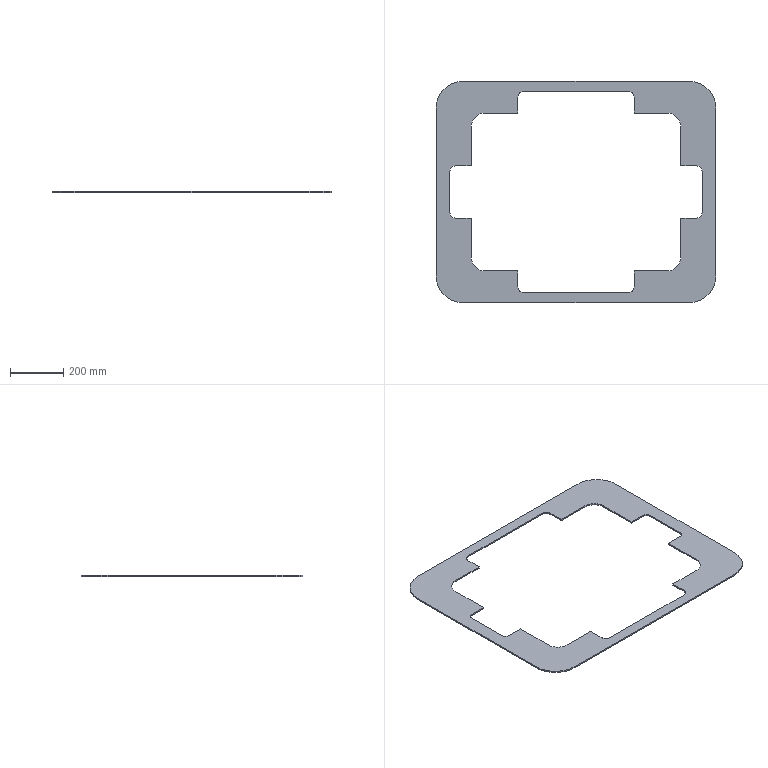Part | NX | features BREP 1 | 1 solid | 42 faces | box 1050 x 830 x 5 mm | volume 1500882 mm3 | plane 26 | cylinder 16 | commonest cylinder face diameters 40 x8 100 x4 200 x4
STEP:
#1=CARTESIAN_POINT('',(817.695,560.835,5.));
#2=VERTEX_POINT('',#1);
#3=CARTESIAN_POINT('',(817.695,560.835,0.));
#4=VERTEX_POINT('',#3);
#5=CARTESIAN_POINT('',(817.695,560.835,44.));
#6=DIRECTION('',(0.,0.,-1.));
#7=VECTOR('',#6,1000.);
#8=LINE('',#5,#7);
#9=EDGE_CURVE('',#2,#4,#8,.T.);
#10=ORIENTED_EDGE('',*,*,#9,.T.);
#11=CARTESIAN_POINT('',(817.695,412.627,0.));
#12=VERTEX_POINT('',#11);
#13=CARTESIAN_POINT('',(817.695,630.,0.));
#14=DIRECTION('',(0.,1.,0.));
#15=VECTOR('',#14,1000.);
#16=LINE('',#13,#15);
#17=EDGE_CURVE('',#12,#4,#16,.T.);
#18=ORIENTED_EDGE('',*,*,#17,.F.);
#19=CARTESIAN_POINT('',(817.695,412.627,5.));
#20=VERTEX_POINT('',#19);
#21=CARTESIAN_POINT('',(817.695,412.627,44.));
#22=DIRECTION('',(0.,0.,-1.));
#23=VECTOR('',#22,1000.);
#24=LINE('',#21,#23);
#25=EDGE_CURVE('',#20,#12,#24,.T.);
#26=ORIENTED_EDGE('',*,*,#25,.F.);
#27=CARTESIAN_POINT('',(817.695,630.,5.));
#28=DIRECTION('',(0.,-1.,0.));
#29=VECTOR('',#28,1000.);
#30=LINE('',#27,#29);
#31=EDGE_CURVE('',#2,#20,#30,.T.);
#32=ORIENTED_EDGE('',*,*,#31,.F.);
#33=EDGE_LOOP('',(#10,#18,#26,#32));
#34=FACE_BOUND('',#33,.T.);
#35=CARTESIAN_POINT('',(817.695,467.627,44.));
#36=DIRECTION('',(-1.,0.,0.));
#37=DIRECTION('',(0.,-1.,0.));
#38=AXIS2_PLACEMENT_3D('',#35,#36,#37);
#39=PLANE('',#38);
#40=ADVANCED_FACE('',(#34),#39,.T.);
#41=CARTESIAN_POINT('',(642.627,610.835,0.));
#42=VERTEX_POINT('',#41);
#43=CARTESIAN_POINT('',(642.627,610.835,5.));
#44=VERTEX_POINT('',#43);
#45=CARTESIAN_POINT('',(642.627,610.835,44.));
#46=DIRECTION('',(0.,0.,1.));
#47=VECTOR('',#46,1000.);
#48=LINE('',#45,#47);
#49=EDGE_CURVE('',#42,#44,#48,.T.);
#50=ORIENTED_EDGE('',*,*,#49,.F.);
#51=CARTESIAN_POINT('',(767.695,610.835,0.));
#52=VERTEX_POINT('',#51);
#53=CARTESIAN_POINT('',(850.,610.835,0.));
#54=DIRECTION('',(-1.,0.,0.));
#55=VECTOR('',#54,1000.);
#56=LINE('',#53,#55);
#57=EDGE_CURVE('',#52,#42,#56,.T.);
#58=ORIENTED_EDGE('',*,*,#57,.F.);
#59=CARTESIAN_POINT('',(767.695,610.835,5.));
#60=VERTEX_POINT('',#59);
#61=CARTESIAN_POINT('',(767.695,610.835,44.));
#62=DIRECTION('',(0.,0.,-1.));
#63=VECTOR('',#62,1000.);
#64=LINE('',#61,#63);
#65=EDGE_CURVE('',#60,#52,#64,.T.);
#66=ORIENTED_EDGE('',*,*,#65,.F.);
#67=CARTESIAN_POINT('',(850.,610.835,5.));
#68=DIRECTION('',(1.,0.,0.));
#69=VECTOR('',#68,1000.);
#70=LINE('',#67,#69);
#71=EDGE_CURVE('',#44,#60,#70,.T.);
#72=ORIENTED_EDGE('',*,*,#71,.F.);
#73=EDGE_LOOP('',(#50,#58,#66,#72));
#74=FACE_BOUND('',#73,.T.);
#75=CARTESIAN_POINT('',(687.627,610.835,44.));
#76=DIRECTION('',(0.,-1.,0.));
#77=DIRECTION('',(1.,0.,0.));
#78=AXIS2_PLACEMENT_3D('',#75,#76,#77);
#79=PLANE('',#78);
#80=ADVANCED_FACE('',(#74),#79,.T.);
#81=ORIENTED_EDGE('',*,*,#65,.T.);
#82=CARTESIAN_POINT('',(767.695,560.835,0.));
#83=DIRECTION('',(0.,0.,1.));
#84=DIRECTION('',(-1.,0.,0.));
#85=AXIS2_PLACEMENT_3D('',#82,#83,#84);
#86=CIRCLE('',#85,50.);
#87=EDGE_CURVE('',#4,#52,#86,.T.);
#88=ORIENTED_EDGE('',*,*,#87,.F.);
#89=ORIENTED_EDGE('',*,*,#9,.F.);
#90=CARTESIAN_POINT('',(767.695,560.835,5.));
#91=DIRECTION('',(0.,0.,1.));
#92=DIRECTION('',(-1.,0.,0.));
#93=AXIS2_PLACEMENT_3D('',#90,#91,#92);
#94=CIRCLE('',#93,50.);
#95=EDGE_CURVE('',#2,#60,#94,.T.);
#96=ORIENTED_EDGE('',*,*,#95,.T.);
#97=EDGE_LOOP('',(#81,#88,#89,#96));
#98=FACE_BOUND('',#97,.T.);
#99=CARTESIAN_POINT('',(767.695,560.835,44.));
#100=DIRECTION('',(0.,0.,-1.));
#101=DIRECTION('',(-1.,0.,0.));
#102=AXIS2_PLACEMENT_3D('',#99,#100,#101);
#103=CYLINDRICAL_SURFACE('',#102,50.);
#104=ADVANCED_FACE('',(#98),#103,.F.);
#105=CARTESIAN_POINT('',(642.627,-40.835,0.));
#106=VERTEX_POINT('',#105);
#107=CARTESIAN_POINT('',(642.627,19.165,0.));
#108=VERTEX_POINT('',#107);
#109=CARTESIAN_POINT('',(642.627,-60.835,0.));
#110=DIRECTION('',(0.,1.,0.));
#111=VECTOR('',#110,1000.);
#112=LINE('',#109,#111);
#113=EDGE_CURVE('',#106,#108,#112,.T.);
#114=ORIENTED_EDGE('',*,*,#113,.F.);
#115=CARTESIAN_POINT('',(642.627,-40.835,5.));
#116=VERTEX_POINT('',#115);
#117=CARTESIAN_POINT('',(642.627,-40.835,5.));
#118=DIRECTION('',(0.,0.,1.));
#119=VECTOR('',#118,1000.);
#120=LINE('',#117,#119);
#121=EDGE_CURVE('',#106,#116,#120,.T.);
#122=ORIENTED_EDGE('',*,*,#121,.T.);
#123=CARTESIAN_POINT('',(642.627,19.165,5.));
#124=VERTEX_POINT('',#123);
#125=CARTESIAN_POINT('',(642.627,-60.835,5.));
#126=DIRECTION('',(0.,1.,0.));
#127=VECTOR('',#126,1000.);
#128=LINE('',#125,#127);
#129=EDGE_CURVE('',#116,#124,#128,.T.);
#130=ORIENTED_EDGE('',*,*,#129,.T.);
#131=CARTESIAN_POINT('',(642.627,19.165,44.));
#132=DIRECTION('',(0.,0.,-1.));
#133=VECTOR('',#132,1000.);
#134=LINE('',#131,#133);
#135=EDGE_CURVE('',#124,#108,#134,.T.);
#136=ORIENTED_EDGE('',*,*,#135,.T.);
#137=EDGE_LOOP('',(#114,#122,#130,#136));
#138=FACE_BOUND('',#137,.T.);
#139=CARTESIAN_POINT('',(642.627,-60.835,0.));
#140=DIRECTION('',(1.,0.,0.));
#141=DIRECTION('',(0.,-1.,0.));
#142=AXIS2_PLACEMENT_3D('',#139,#140,#141);
#143=PLANE('',#142);
#144=ADVANCED_FACE('',(#138),#143,.F.);
#145=CARTESIAN_POINT('',(227.373,-60.835,5.));
#146=VERTEX_POINT('',#145);
#147=CARTESIAN_POINT('',(622.627,-60.835,5.));
#148=VERTEX_POINT('',#147);
#149=CARTESIAN_POINT('',(167.373,-60.835,5.));
#150=DIRECTION('',(1.,0.,0.));
#151=VECTOR('',#150,1000.);
#152=LINE('',#149,#151);
#153=EDGE_CURVE('',#146,#148,#152,.T.);
#154=ORIENTED_EDGE('',*,*,#153,.T.);
#155=CARTESIAN_POINT('',(622.627,-60.835,0.));
#156=VERTEX_POINT('',#155);
#157=CARTESIAN_POINT('',(622.627,-60.835,0.));
#158=DIRECTION('',(0.,0.,-1.));
#159=VECTOR('',#158,1000.);
#160=LINE('',#157,#159);
#161=EDGE_CURVE('',#148,#156,#160,.T.);
#162=ORIENTED_EDGE('',*,*,#161,.T.);
#163=CARTESIAN_POINT('',(227.373,-60.835,0.));
#164=VERTEX_POINT('',#163);
#165=CARTESIAN_POINT('',(167.373,-60.835,0.));
#166=DIRECTION('',(1.,0.,0.));
#167=VECTOR('',#166,1000.);
#168=LINE('',#165,#167);
#169=EDGE_CURVE('',#164,#156,#168,.T.);
#170=ORIENTED_EDGE('',*,*,#169,.F.);
#171=CARTESIAN_POINT('',(227.373,-60.835,5.));
#172=DIRECTION('',(0.,0.,1.));
#173=VECTOR('',#172,1000.);
#174=LINE('',#171,#173);
#175=EDGE_CURVE('',#164,#146,#174,.T.);
#176=ORIENTED_EDGE('',*,*,#175,.T.);
#177=EDGE_LOOP('',(#154,#162,#170,#176));
#178=FACE_BOUND('',#177,.T.);
#179=CARTESIAN_POINT('',(167.373,-60.835,0.));
#180=DIRECTION('',(0.,-1.,0.));
#181=DIRECTION('',(-1.,0.,0.));
#182=AXIS2_PLACEMENT_3D('',#179,#180,#181);
#183=PLANE('',#182);
#184=ADVANCED_FACE('',(#178),#183,.F.);
#185=CARTESIAN_POINT('',(207.373,19.165,5.));
#186=VERTEX_POINT('',#185);
#187=CARTESIAN_POINT('',(207.373,-40.835,5.));
#188=VERTEX_POINT('',#187);
#189=CARTESIAN_POINT('',(207.373,167.373,5.));
#190=DIRECTION('',(0.,-1.,0.));
#191=VECTOR('',#190,1000.);
#192=LINE('',#189,#191);
#193=EDGE_CURVE('',#186,#188,#192,.T.);
#194=ORIENTED_EDGE('',*,*,#193,.T.);
#195=CARTESIAN_POINT('',(207.373,-40.835,0.));
#196=VERTEX_POINT('',#195);
#197=CARTESIAN_POINT('',(207.373,-40.835,0.));
#198=DIRECTION('',(0.,0.,-1.));
#199=VECTOR('',#198,1000.);
#200=LINE('',#197,#199);
#201=EDGE_CURVE('',#188,#196,#200,.T.);
#202=ORIENTED_EDGE('',*,*,#201,.T.);
#203=CARTESIAN_POINT('',(207.373,19.165,0.));
#204=VERTEX_POINT('',#203);
#205=CARTESIAN_POINT('',(207.373,167.373,0.));
#206=DIRECTION('',(0.,-1.,0.));
#207=VECTOR('',#206,1000.);
#208=LINE('',#205,#207);
#209=EDGE_CURVE('',#204,#196,#208,.T.);
#210=ORIENTED_EDGE('',*,*,#209,.F.);
#211=CARTESIAN_POINT('',(207.373,19.165,44.));
#212=DIRECTION('',(0.,0.,1.));
#213=VECTOR('',#212,1000.);
#214=LINE('',#211,#213);
#215=EDGE_CURVE('',#204,#186,#214,.T.);
#216=ORIENTED_EDGE('',*,*,#215,.T.);
#217=EDGE_LOOP('',(#194,#202,#210,#216));
#218=FACE_BOUND('',#217,.T.);
#219=CARTESIAN_POINT('',(207.373,167.373,0.));
#220=DIRECTION('',(-1.,0.,0.));
#221=DIRECTION('',(0.,1.,0.));
#222=AXIS2_PLACEMENT_3D('',#219,#220,#221);
#223=PLANE('',#222);
#224=ADVANCED_FACE('',(#218),#223,.F.);
#225=ORIENTED_EDGE('',*,*,#215,.F.);
#226=CARTESIAN_POINT('',(82.305,19.165,0.));
#227=VERTEX_POINT('',#226);
#228=CARTESIAN_POINT('',(0.,19.165,0.));
#229=DIRECTION('',(1.,0.,0.));
#230=VECTOR('',#229,1000.);
#231=LINE('',#228,#230);
#232=EDGE_CURVE('',#227,#204,#231,.T.);
#233=ORIENTED_EDGE('',*,*,#232,.F.);
#234=CARTESIAN_POINT('',(82.305,19.165,5.));
#235=VERTEX_POINT('',#234);
#236=CARTESIAN_POINT('',(82.305,19.165,44.));
#237=DIRECTION('',(0.,0.,-1.));
#238=VECTOR('',#237,1000.);
#239=LINE('',#236,#238);
#240=EDGE_CURVE('',#235,#227,#239,.T.);
#241=ORIENTED_EDGE('',*,*,#240,.F.);
#242=CARTESIAN_POINT('',(0.,19.165,5.));
#243=DIRECTION('',(-1.,0.,0.));
#244=VECTOR('',#243,1000.);
#245=LINE('',#242,#244);
#246=EDGE_CURVE('',#186,#235,#245,.T.);
#247=ORIENTED_EDGE('',*,*,#246,.F.);
#248=EDGE_LOOP('',(#225,#233,#241,#247));
#249=FACE_BOUND('',#248,.T.);
#250=CARTESIAN_POINT('',(162.373,19.165,44.));
#251=DIRECTION('',(0.,1.,0.));
#252=DIRECTION('',(-1.,0.,0.));
#253=AXIS2_PLACEMENT_3D('',#250,#251,#252);
#254=PLANE('',#253);
#255=ADVANCED_FACE('',(#249),#254,.T.);
#256=ORIENTED_EDGE('',*,*,#240,.T.);
#257=CARTESIAN_POINT('',(32.305,69.165,0.));
#258=VERTEX_POINT('',#257);
#259=CARTESIAN_POINT('',(82.305,69.165,0.));
#260=DIRECTION('',(0.,0.,1.));
#261=DIRECTION('',(-1.,0.,0.));
#262=AXIS2_PLACEMENT_3D('',#259,#260,#261);
#263=CIRCLE('',#262,50.);
#264=EDGE_CURVE('',#258,#227,#263,.T.);
#265=ORIENTED_EDGE('',*,*,#264,.F.);
#266=CARTESIAN_POINT('',(32.305,69.165,5.));
#267=VERTEX_POINT('',#266);
#268=CARTESIAN_POINT('',(32.305,69.165,44.));
#269=DIRECTION('',(0.,0.,-1.));
#270=VECTOR('',#269,1000.);
#271=LINE('',#268,#270);
#272=EDGE_CURVE('',#267,#258,#271,.T.);
#273=ORIENTED_EDGE('',*,*,#272,.F.);
#274=CARTESIAN_POINT('',(82.305,69.165,5.));
#275=DIRECTION('',(0.,0.,1.));
#276=DIRECTION('',(-1.,0.,0.));
#277=AXIS2_PLACEMENT_3D('',#274,#275,#276);
#278=CIRCLE('',#277,50.);
#279=EDGE_CURVE('',#267,#235,#278,.T.);
#280=ORIENTED_EDGE('',*,*,#279,.T.);
#281=EDGE_LOOP('',(#256,#265,#273,#280));
#282=FACE_BOUND('',#281,.T.);
#283=CARTESIAN_POINT('',(82.305,69.165,44.));
#284=DIRECTION('',(0.,0.,-1.));
#285=DIRECTION('',(1.,0.,0.));
#286=AXIS2_PLACEMENT_3D('',#283,#284,#285);
#287=CYLINDRICAL_SURFACE('',#286,50.);
#288=ADVANCED_FACE('',(#282),#287,.F.);
#289=ORIENTED_EDGE('',*,*,#272,.T.);
#290=CARTESIAN_POINT('',(32.305,217.373,0.));
#291=VERTEX_POINT('',#290);
#292=CARTESIAN_POINT('',(32.305,0.,0.));
#293=DIRECTION('',(0.,-1.,0.));
#294=VECTOR('',#293,1000.);
#295=LINE('',#292,#294);
#296=EDGE_CURVE('',#291,#258,#295,.T.);
#297=ORIENTED_EDGE('',*,*,#296,.F.);
#298=CARTESIAN_POINT('',(32.305,217.373,5.));
#299=VERTEX_POINT('',#298);
#300=CARTESIAN_POINT('',(32.305,217.373,44.));
#301=DIRECTION('',(0.,0.,-1.));
#302=VECTOR('',#301,1000.);
#303=LINE('',#300,#302);
#304=EDGE_CURVE('',#299,#291,#303,.T.);
#305=ORIENTED_EDGE('',*,*,#304,.F.);
#306=CARTESIAN_POINT('',(32.305,0.,5.));
#307=DIRECTION('',(0.,1.,0.));
#308=VECTOR('',#307,1000.);
#309=LINE('',#306,#308);
#310=EDGE_CURVE('',#267,#299,#309,.T.);
#311=ORIENTED_EDGE('',*,*,#310,.F.);
#312=EDGE_LOOP('',(#289,#297,#305,#311));
#313=FACE_BOUND('',#312,.T.);
#314=CARTESIAN_POINT('',(32.305,162.373,44.));
#315=DIRECTION('',(1.,0.,0.));
#316=DIRECTION('',(0.,1.,0.));
#317=AXIS2_PLACEMENT_3D('',#314,#315,#316);
#318=PLANE('',#317);
#319=ADVANCED_FACE('',(#313),#318,.T.);
#320=CARTESIAN_POINT('',(-27.695,217.373,0.));
#321=VERTEX_POINT('',#320);
#322=CARTESIAN_POINT('',(-47.695,217.373,0.));
#323=DIRECTION('',(1.,0.,0.));
#324=VECTOR('',#323,1000.);
#325=LINE('',#322,#324);
#326=EDGE_CURVE('',#321,#291,#325,.T.);
#327=ORIENTED_EDGE('',*,*,#326,.F.);
#328=CARTESIAN_POINT('',(-27.695,217.373,5.));
#329=VERTEX_POINT('',#328);
#330=CARTESIAN_POINT('',(-27.695,217.373,5.));
#331=DIRECTION('',(0.,0.,1.));
#332=VECTOR('',#331,1000.);
#333=LINE('',#330,#332);
#334=EDGE_CURVE('',#321,#329,#333,.T.);
#335=ORIENTED_EDGE('',*,*,#334,.T.);
#336=CARTESIAN_POINT('',(-47.695,217.373,5.));
#337=DIRECTION('',(1.,0.,0.));
#338=VECTOR('',#337,1000.);
#339=LINE('',#336,#338);
#340=EDGE_CURVE('',#329,#299,#339,.T.);
#341=ORIENTED_EDGE('',*,*,#340,.T.);
#342=ORIENTED_EDGE('',*,*,#304,.T.);
#343=EDGE_LOOP('',(#327,#335,#341,#342));
#344=FACE_BOUND('',#343,.T.);
#345=CARTESIAN_POINT('',(-47.695,217.373,0.));
#346=DIRECTION('',(0.,-1.,0.));
#347=DIRECTION('',(-1.,0.,0.));
#348=AXIS2_PLACEMENT_3D('',#345,#346,#347);
#349=PLANE('',#348);
#350=ADVANCED_FACE('',(#344),#349,.F.);
#351=CARTESIAN_POINT('',(-47.695,392.627,0.));
#352=VERTEX_POINT('',#351);
#353=CARTESIAN_POINT('',(-47.695,237.373,0.));
#354=VERTEX_POINT('',#353);
#355=CARTESIAN_POINT('',(-47.695,462.627,0.));
#356=DIRECTION('',(0.,-1.,0.));
#357=VECTOR('',#356,1000.);
#358=LINE('',#355,#357);
#359=EDGE_CURVE('',#352,#354,#358,.T.);
#360=ORIENTED_EDGE('',*,*,#359,.F.);
#361=CARTESIAN_POINT('',(-47.695,392.627,5.));
#362=VERTEX_POINT('',#361);
#363=CARTESIAN_POINT('',(-47.695,392.627,5.));
#364=DIRECTION('',(0.,0.,1.));
#365=VECTOR('',#364,1000.);
#366=LINE('',#363,#365);
#367=EDGE_CURVE('',#352,#362,#366,.T.);
#368=ORIENTED_EDGE('',*,*,#367,.T.);
#369=CARTESIAN_POINT('',(-47.695,237.373,5.));
#370=VERTEX_POINT('',#369);
#371=CARTESIAN_POINT('',(-47.695,462.627,5.));
#372=DIRECTION('',(0.,-1.,0.));
#373=VECTOR('',#372,1000.);
#374=LINE('',#371,#373);
#375=EDGE_CURVE('',#362,#370,#374,.T.);
#376=ORIENTED_EDGE('',*,*,#375,.T.);
#377=CARTESIAN_POINT('',(-47.695,237.373,0.));
#378=DIRECTION('',(0.,0.,-1.));
#379=VECTOR('',#378,1000.);
#380=LINE('',#377,#379);
#381=EDGE_CURVE('',#370,#354,#380,.T.);
#382=ORIENTED_EDGE('',*,*,#381,.T.);
#383=EDGE_LOOP('',(#360,#368,#376,#382));
#384=FACE_BOUND('',#383,.T.);
#385=CARTESIAN_POINT('',(-47.695,462.627,0.));
#386=DIRECTION('',(-1.,0.,0.));
#387=DIRECTION('',(0.,1.,0.));
#388=AXIS2_PLACEMENT_3D('',#385,#386,#387);
#389=PLANE('',#388);
#390=ADVANCED_FACE('',(#384),#389,.F.);
#391=CARTESIAN_POINT('',(32.305,412.627,5.));
#392=VERTEX_POINT('',#391);
#393=CARTESIAN_POINT('',(-27.695,412.627,5.));
#394=VERTEX_POINT('',#393);
#395=CARTESIAN_POINT('',(167.373,412.627,5.));
#396=DIRECTION('',(-1.,0.,0.));
#397=VECTOR('',#396,1000.);
#398=LINE('',#395,#397);
#399=EDGE_CURVE('',#392,#394,#398,.T.);
#400=ORIENTED_EDGE('',*,*,#399,.T.);
#401=CARTESIAN_POINT('',(-27.695,412.627,0.));
#402=VERTEX_POINT('',#401);
#403=CARTESIAN_POINT('',(-27.695,412.627,0.));
#404=DIRECTION('',(0.,0.,-1.));
#405=VECTOR('',#404,1000.);
#406=LINE('',#403,#405);
#407=EDGE_CURVE('',#394,#402,#406,.T.);
#408=ORIENTED_EDGE('',*,*,#407,.T.);
#409=CARTESIAN_POINT('',(32.305,412.627,0.));
#410=VERTEX_POINT('',#409);
#411=CARTESIAN_POINT('',(167.373,412.627,0.));
#412=DIRECTION('',(-1.,0.,0.));
#413=VECTOR('',#412,1000.);
#414=LINE('',#411,#413);
#415=EDGE_CURVE('',#410,#402,#414,.T.);
#416=ORIENTED_EDGE('',*,*,#415,.F.);
#417=CARTESIAN_POINT('',(32.305,412.627,0.));
#418=DIRECTION('',(0.,0.,-1.));
#419=VECTOR('',#418,1000.);
#420=LINE('',#417,#419);
#421=EDGE_CURVE('',#392,#410,#420,.T.);
#422=ORIENTED_EDGE('',*,*,#421,.F.);
#423=EDGE_LOOP('',(#400,#408,#416,#422));
#424=FACE_BOUND('',#423,.T.);
#425=CARTESIAN_POINT('',(167.373,412.627,0.));
#426=DIRECTION('',(0.,1.,0.));
#427=DIRECTION('',(1.,0.,0.));
#428=AXIS2_PLACEMENT_3D('',#425,#426,#427);
#429=PLANE('',#428);
#430=ADVANCED_FACE('',(#424),#429,.F.);
#431=CARTESIAN_POINT('',(32.305,560.835,0.));
#432=VERTEX_POINT('',#431);
#433=CARTESIAN_POINT('',(32.305,560.835,5.));
#434=VERTEX_POINT('',#433);
#435=CARTESIAN_POINT('',(32.305,560.835,44.));
#436=DIRECTION('',(0.,0.,1.));
#437=VECTOR('',#436,1000.);
#438=LINE('',#435,#437);
#439=EDGE_CURVE('',#432,#434,#438,.T.);
#440=ORIENTED_EDGE('',*,*,#439,.T.);
#441=CARTESIAN_POINT('',(32.305,630.,5.));
#442=DIRECTION('',(0.,-1.,0.));
#443=VECTOR('',#442,1000.);
#444=LINE('',#441,#443);
#445=EDGE_CURVE('',#434,#392,#444,.T.);
#446=ORIENTED_EDGE('',*,*,#445,.T.);
#447=ORIENTED_EDGE('',*,*,#421,.T.);
#448=CARTESIAN_POINT('',(32.305,630.,0.));
#449=DIRECTION('',(0.,-1.,0.));
#450=VECTOR('',#449,1000.);
#451=LINE('',#448,#450);
#452=EDGE_CURVE('',#432,#410,#451,.T.);
#453=ORIENTED_EDGE('',*,*,#452,.F.);
#454=EDGE_LOOP('',(#440,#446,#447,#453));
#455=FACE_BOUND('',#454,.T.);
#456=CARTESIAN_POINT('',(32.305,467.627,44.));
#457=DIRECTION('',(1.,0.,0.));
#458=DIRECTION('',(0.,-1.,0.));
#459=AXIS2_PLACEMENT_3D('',#456,#457,#458);
#460=PLANE('',#459);
#461=ADVANCED_FACE('',(#455),#460,.T.);
#462=CARTESIAN_POINT('',(82.305,610.835,0.));
#463=VERTEX_POINT('',#462);
#464=CARTESIAN_POINT('',(82.305,610.835,5.));
#465=VERTEX_POINT('',#464);
#466=CARTESIAN_POINT('',(82.305,610.835,44.));
#467=DIRECTION('',(0.,0.,1.));
#468=VECTOR('',#467,1000.);
#469=LINE('',#466,#468);
#470=EDGE_CURVE('',#463,#465,#469,.T.);
#471=ORIENTED_EDGE('',*,*,#470,.T.);
#472=CARTESIAN_POINT('',(82.305,560.835,5.));
#473=DIRECTION('',(0.,0.,1.));
#474=DIRECTION('',(-1.,0.,0.));
#475=AXIS2_PLACEMENT_3D('',#472,#473,#474);
#476=CIRCLE('',#475,50.);
#477=EDGE_CURVE('',#465,#434,#476,.T.);
#478=ORIENTED_EDGE('',*,*,#477,.T.);
#479=ORIENTED_EDGE('',*,*,#439,.F.);
#480=CARTESIAN_POINT('',(82.305,560.835,0.));
#481=DIRECTION('',(0.,0.,1.));
#482=DIRECTION('',(-1.,0.,0.));
#483=AXIS2_PLACEMENT_3D('',#480,#481,#482);
#484=CIRCLE('',#483,50.);
#485=EDGE_CURVE('',#463,#432,#484,.T.);
#486=ORIENTED_EDGE('',*,*,#485,.F.);
#487=EDGE_LOOP('',(#471,#478,#479,#486));
#488=FACE_BOUND('',#487,.T.);
#489=CARTESIAN_POINT('',(82.305,560.835,44.));
#490=DIRECTION('',(0.,0.,-1.));
#491=DIRECTION('',(1.,0.,0.));
#492=AXIS2_PLACEMENT_3D('',#489,#490,#491);
#493=CYLINDRICAL_SURFACE('',#492,50.);
#494=ADVANCED_FACE('',(#488),#493,.F.);
#495=CARTESIAN_POINT('',(207.373,610.835,0.));
#496=VERTEX_POINT('',#495);
#497=CARTESIAN_POINT('',(207.373,610.835,5.));
#498=VERTEX_POINT('',#497);
#499=CARTESIAN_POINT('',(207.373,610.835,0.));
#500=DIRECTION('',(0.,0.,1.));
#501=VECTOR('',#500,1000.);
#502=LINE('',#499,#501);
#503=EDGE_CURVE('',#496,#498,#502,.T.);
#504=ORIENTED_EDGE('',*,*,#503,.T.);
#505=CARTESIAN_POINT('',(0.,610.835,5.));
#506=DIRECTION('',(-1.,0.,0.));
#507=VECTOR('',#506,1000.);
#508=LINE('',#505,#507);
#509=EDGE_CURVE('',#498,#465,#508,.T.);
#510=ORIENTED_EDGE('',*,*,#509,.T.);
#511=ORIENTED_EDGE('',*,*,#470,.F.);
#512=CARTESIAN_POINT('',(0.,610.835,0.));
#513=DIRECTION('',(-1.,0.,0.));
#514=VECTOR('',#513,1000.);
#515=LINE('',#512,#514);
#516=EDGE_CURVE('',#496,#463,#515,.T.);
#517=ORIENTED_EDGE('',*,*,#516,.F.);
#518=EDGE_LOOP('',(#504,#510,#511,#517));
#519=FACE_BOUND('',#518,.T.);
#520=CARTESIAN_POINT('',(162.373,610.835,44.));
#521=DIRECTION('',(0.,-1.,0.));
#522=DIRECTION('',(-1.,0.,0.));
#523=AXIS2_PLACEMENT_3D('',#520,#521,#522);
#524=PLANE('',#523);
#525=ADVANCED_FACE('',(#519),#524,.T.);
#526=CARTESIAN_POINT('',(207.373,670.835,0.));
#527=VERTEX_POINT('',#526);
#528=CARTESIAN_POINT('',(207.373,690.835,0.));
#529=DIRECTION('',(0.,-1.,0.));
#530=VECTOR('',#529,1000.);
#531=LINE('',#528,#530);
#532=EDGE_CURVE('',#527,#496,#531,.T.);
#533=ORIENTED_EDGE('',*,*,#532,.F.);
#534=CARTESIAN_POINT('',(207.373,670.835,5.));
#535=VERTEX_POINT('',#534);
#536=CARTESIAN_POINT('',(207.373,670.835,5.));
#537=DIRECTION('',(0.,0.,1.));
#538=VECTOR('',#537,1000.);
#539=LINE('',#536,#538);
#540=EDGE_CURVE('',#527,#535,#539,.T.);
#541=ORIENTED_EDGE('',*,*,#540,.T.);
#542=CARTESIAN_POINT('',(207.373,690.835,5.));
#543=DIRECTION('',(0.,-1.,0.));
#544=VECTOR('',#543,1000.);
#545=LINE('',#542,#544);
#546=EDGE_CURVE('',#535,#498,#545,.T.);
#547=ORIENTED_EDGE('',*,*,#546,.T.);
#548=ORIENTED_EDGE('',*,*,#503,.F.);
#549=EDGE_LOOP('',(#533,#541,#547,#548));
#550=FACE_BOUND('',#549,.T.);
#551=CARTESIAN_POINT('',(207.373,690.835,0.));
#552=DIRECTION('',(-1.,0.,0.));
#553=DIRECTION('',(0.,1.,0.));
#554=AXIS2_PLACEMENT_3D('',#551,#552,#553);
#555=PLANE('',#554);
#556=ADVANCED_FACE('',(#550),#555,.F.);
#557=CARTESIAN_POINT('',(622.627,690.835,5.));
#558=VERTEX_POINT('',#557);
#559=CARTESIAN_POINT('',(227.373,690.835,5.));
#560=VERTEX_POINT('',#559);
#561=CARTESIAN_POINT('',(682.627,690.835,5.));
#562=DIRECTION('',(-1.,0.,0.));
#563=VECTOR('',#562,1000.);
#564=LINE('',#561,#563);
#565=EDGE_CURVE('',#558,#560,#564,.T.);
#566=ORIENTED_EDGE('',*,*,#565,.T.);
#567=CARTESIAN_POINT('',(227.373,690.835,0.));
#568=VERTEX_POINT('',#567);
#569=CARTESIAN_POINT('',(227.373,690.835,0.));
#570=DIRECTION('',(0.,0.,-1.));
#571=VECTOR('',#570,1000.);
#572=LINE('',#569,#571);
#573=EDGE_CURVE('',#560,#568,#572,.T.);
#574=ORIENTED_EDGE('',*,*,#573,.T.);
#575=CARTESIAN_POINT('',(622.627,690.835,0.));
#576=VERTEX_POINT('',#575);
#577=CARTESIAN_POINT('',(682.627,690.835,0.));
#578=DIRECTION('',(-1.,0.,0.));
#579=VECTOR('',#578,1000.);
#580=LINE('',#577,#579);
#581=EDGE_CURVE('',#576,#568,#580,.T.);
#582=ORIENTED_EDGE('',*,*,#581,.F.);
#583=CARTESIAN_POINT('',(622.627,690.835,5.));
#584=DIRECTION('',(0.,0.,1.));
#585=VECTOR('',#584,1000.);
#586=LINE('',#583,#585);
#587=EDGE_CURVE('',#576,#558,#586,.T.);
#588=ORIENTED_EDGE('',*,*,#587,.T.);
#589=EDGE_LOOP('',(#566,#574,#582,#588));
#590=FACE_BOUND('',#589,.T.);
#591=CARTESIAN_POINT('',(682.627,690.835,0.));
#592=DIRECTION('',(0.,1.,0.));
#593=DIRECTION('',(1.,0.,0.));
#594=AXIS2_PLACEMENT_3D('',#591,#592,#593);
#595=PLANE('',#594);
#596=ADVANCED_FACE('',(#590),#595,.F.);
#597=CARTESIAN_POINT('',(642.627,670.835,5.));
#598=VERTEX_POINT('',#597);
#599=CARTESIAN_POINT('',(642.627,462.627,5.));
#600=DIRECTION('',(0.,1.,0.));
#601=VECTOR('',#600,1000.);
#602=LINE('',#599,#601);
#603=EDGE_CURVE('',#44,#598,#602,.T.);
#604=ORIENTED_EDGE('',*,*,#603,.T.);
#605=CARTESIAN_POINT('',(642.627,670.835,0.));
#606=VERTEX_POINT('',#605);
#607=CARTESIAN_POINT('',(642.627,670.835,0.));
#608=DIRECTION('',(0.,0.,-1.));
#609=VECTOR('',#608,1000.);
#610=LINE('',#607,#609);
#611=EDGE_CURVE('',#598,#606,#610,.T.);
#612=ORIENTED_EDGE('',*,*,#611,.T.);
#613=CARTESIAN_POINT('',(642.627,462.627,0.));
#614=DIRECTION('',(0.,1.,0.));
#615=VECTOR('',#614,1000.);
#616=LINE('',#613,#615);
#617=EDGE_CURVE('',#42,#606,#616,.T.);
#618=ORIENTED_EDGE('',*,*,#617,.F.);
#619=ORIENTED_EDGE('',*,*,#49,.T.);
#620=EDGE_LOOP('',(#604,#612,#618,#619));
#621=FACE_BOUND('',#620,.T.);
#622=CARTESIAN_POINT('',(642.627,462.627,0.));
#623=DIRECTION('',(1.,0.,0.));
#624=DIRECTION('',(0.,-1.,0.));
#625=AXIS2_PLACEMENT_3D('',#622,#623,#624);
#626=PLANE('',#625);
#627=ADVANCED_FACE('',(#621),#626,.F.);
#628=CARTESIAN_POINT('',(877.695,412.627,0.));
#629=VERTEX_POINT('',#628);
#630=CARTESIAN_POINT('',(897.695,412.627,0.));
#631=DIRECTION('',(-1.,0.,0.));
#632=VECTOR('',#631,1000.);
#633=LINE('',#630,#632);
#634=EDGE_CURVE('',#629,#12,#633,.T.);
#635=ORIENTED_EDGE('',*,*,#634,.F.);
#636=CARTESIAN_POINT('',(877.695,412.627,5.));
#637=VERTEX_POINT('',#636);
#638=CARTESIAN_POINT('',(877.695,412.627,5.));
#639=DIRECTION('',(0.,0.,1.));
#640=VECTOR('',#639,1000.);
#641=LINE('',#638,#640);
#642=EDGE_CURVE('',#629,#637,#641,.T.);
#643=ORIENTED_EDGE('',*,*,#642,.T.);
#644=CARTESIAN_POINT('',(897.695,412.627,5.));
#645=DIRECTION('',(-1.,0.,0.));
#646=VECTOR('',#645,1000.);
#647=LINE('',#644,#646);
#648=EDGE_CURVE('',#637,#20,#647,.T.);
#649=ORIENTED_EDGE('',*,*,#648,.T.);
#650=ORIENTED_EDGE('',*,*,#25,.T.);
#651=EDGE_LOOP('',(#635,#643,#649,#650));
#652=FACE_BOUND('',#651,.T.);
#653=CARTESIAN_POINT('',(897.695,412.627,0.));
#654=DIRECTION('',(0.,1.,0.));
#655=DIRECTION('',(1.,0.,0.));
#656=AXIS2_PLACEMENT_3D('',#653,#654,#655);
#657=PLANE('',#656);
#658=ADVANCED_FACE('',(#652),#657,.F.);
#659=CARTESIAN_POINT('',(897.695,237.373,5.));
#660=VERTEX_POINT('',#659);
#661=CARTESIAN_POINT('',(897.695,392.627,5.));
#662=VERTEX_POINT('',#661);
#663=CARTESIAN_POINT('',(897.695,167.373,5.));
#664=DIRECTION('',(0.,1.,0.));
#665=VECTOR('',#664,1000.);
#666=LINE('',#663,#665);
#667=EDGE_CURVE('',#660,#662,#666,.T.);
#668=ORIENTED_EDGE('',*,*,#667,.T.);
#669=CARTESIAN_POINT('',(897.695,392.627,0.));
#670=VERTEX_POINT('',#669);
#671=CARTESIAN_POINT('',(897.695,392.627,0.));
#672=DIRECTION('',(0.,0.,-1.));
#673=VECTOR('',#672,1000.);
#674=LINE('',#671,#673);
#675=EDGE_CURVE('',#662,#670,#674,.T.);
#676=ORIENTED_EDGE('',*,*,#675,.T.);
#677=CARTESIAN_POINT('',(897.695,237.373,0.));
#678=VERTEX_POINT('',#677);
#679=CARTESIAN_POINT('',(897.695,167.373,0.));
#680=DIRECTION('',(0.,1.,0.));
#681=VECTOR('',#680,1000.);
#682=LINE('',#679,#681);
#683=EDGE_CURVE('',#678,#670,#682,.T.);
#684=ORIENTED_EDGE('',*,*,#683,.F.);
#685=CARTESIAN_POINT('',(897.695,237.373,5.));
#686=DIRECTION('',(0.,0.,1.));
#687=VECTOR('',#686,1000.);
#688=LINE('',#685,#687);
#689=EDGE_CURVE('',#678,#660,#688,.T.);
#690=ORIENTED_EDGE('',*,*,#689,.T.);
#691=EDGE_LOOP('',(#668,#676,#684,#690));
#692=FACE_BOUND('',#691,.T.);
#693=CARTESIAN_POINT('',(897.695,167.373,0.));
#694=DIRECTION('',(1.,0.,0.));
#695=DIRECTION('',(0.,-1.,0.));
#696=AXIS2_PLACEMENT_3D('',#693,#694,#695);
#697=PLANE('',#696);
#698=ADVANCED_FACE('',(#692),#697,.F.);
#699=CARTESIAN_POINT('',(817.695,217.373,5.));
#700=VERTEX_POINT('',#699);
#701=CARTESIAN_POINT('',(877.695,217.373,5.));
#702=VERTEX_POINT('',#701);
#703=CARTESIAN_POINT('',(682.627,217.373,5.));
#704=DIRECTION('',(1.,0.,0.));
#705=VECTOR('',#704,1000.);
#706=LINE('',#703,#705);
#707=EDGE_CURVE('',#700,#702,#706,.T.);
#708=ORIENTED_EDGE('',*,*,#707,.T.);
#709=CARTESIAN_POINT('',(877.695,217.373,0.));
#710=VERTEX_POINT('',#709);
#711=CARTESIAN_POINT('',(877.695,217.373,0.));
#712=DIRECTION('',(0.,0.,-1.));
#713=VECTOR('',#712,1000.);
#714=LINE('',#711,#713);
#715=EDGE_CURVE('',#702,#710,#714,.T.);
#716=ORIENTED_EDGE('',*,*,#715,.T.);
#717=CARTESIAN_POINT('',(817.695,217.373,0.));
#718=VERTEX_POINT('',#717);
#719=CARTESIAN_POINT('',(682.627,217.373,0.));
#720=DIRECTION('',(1.,0.,0.));
#721=VECTOR('',#720,1000.);
#722=LINE('',#719,#721);
#723=EDGE_CURVE('',#718,#710,#722,.T.);
#724=ORIENTED_EDGE('',*,*,#723,.F.);
#725=CARTESIAN_POINT('',(817.695,217.373,44.));
#726=DIRECTION('',(0.,0.,1.));
#727=VECTOR('',#726,1000.);
#728=LINE('',#725,#727);
#729=EDGE_CURVE('',#718,#700,#728,.T.);
#730=ORIENTED_EDGE('',*,*,#729,.T.);
#731=EDGE_LOOP('',(#708,#716,#724,#730));
#732=FACE_BOUND('',#731,.T.);
#733=CARTESIAN_POINT('',(682.627,217.373,0.));
#734=DIRECTION('',(0.,-1.,0.));
#735=DIRECTION('',(-1.,0.,0.));
#736=AXIS2_PLACEMENT_3D('',#733,#734,#735);
#737=PLANE('',#736);
#738=ADVANCED_FACE('',(#732),#737,.F.);
#739=CARTESIAN_POINT('',(0.,-100.,5.));
#740=VERTEX_POINT('',#739);
#741=CARTESIAN_POINT('',(-100.,0.,5.));
#742=VERTEX_POINT('',#741);
#743=CARTESIAN_POINT('',(0.,0.,5.));
#744=DIRECTION('',(0.,0.,-1.));
#745=DIRECTION('',(0.,1.,0.));
#746=AXIS2_PLACEMENT_3D('',#743,#744,#745);
#747=CIRCLE('',#746,100.);
#748=EDGE_CURVE('',#740,#742,#747,.T.);
#749=ORIENTED_EDGE('',*,*,#748,.T.);
#750=CARTESIAN_POINT('',(-100.,0.,0.));
#751=VERTEX_POINT('',#750);
#752=CARTESIAN_POINT('',(-100.,0.,0.));
#753=DIRECTION('',(0.,0.,1.));
#754=VECTOR('',#753,1000.);
#755=LINE('',#752,#754);
#756=EDGE_CURVE('',#751,#742,#755,.T.);
#757=ORIENTED_EDGE('',*,*,#756,.F.);
#758=CARTESIAN_POINT('',(0.,-100.,0.));
#759=VERTEX_POINT('',#758);
#760=CARTESIAN_POINT('',(0.,0.,0.));
#761=DIRECTION('',(0.,0.,-1.));
#762=DIRECTION('',(0.,1.,0.));
#763=AXIS2_PLACEMENT_3D('',#760,#761,#762);
#764=CIRCLE('',#763,100.);
#765=EDGE_CURVE('',#759,#751,#764,.T.);
#766=ORIENTED_EDGE('',*,*,#765,.F.);
#767=CARTESIAN_POINT('',(0.,-100.,0.));
#768=DIRECTION('',(0.,0.,1.));
#769=VECTOR('',#768,1000.);
#770=LINE('',#767,#769);
#771=EDGE_CURVE('',#759,#740,#770,.T.);
#772=ORIENTED_EDGE('',*,*,#771,.T.);
#773=EDGE_LOOP('',(#749,#757,#766,#772));
#774=FACE_BOUND('',#773,.T.);
#775=CARTESIAN_POINT('',(0.,0.,0.));
#776=DIRECTION('',(0.,0.,1.));
#777=DIRECTION('',(-1.,0.,0.));
#778=AXIS2_PLACEMENT_3D('',#775,#776,#777);
#779=CYLINDRICAL_SURFACE('',#778,100.);
#780=ADVANCED_FACE('',(#774),#779,.T.);
#781=CARTESIAN_POINT('',(850.,-100.,5.));
#782=VERTEX_POINT('',#781);
#783=CARTESIAN_POINT('',(850.,-100.,5.));
#784=DIRECTION('',(-1.,0.,0.));
#785=VECTOR('',#784,1000.);
#786=LINE('',#783,#785);
#787=EDGE_CURVE('',#782,#740,#786,.T.);
#788=ORIENTED_EDGE('',*,*,#787,.T.);
#789=ORIENTED_EDGE('',*,*,#771,.F.);
#790=CARTESIAN_POINT('',(850.,-100.,0.));
#791=VERTEX_POINT('',#790);
#792=CARTESIAN_POINT('',(850.,-100.,0.));
#793=DIRECTION('',(-1.,0.,0.));
#794=VECTOR('',#793,1000.);
#795=LINE('',#792,#794);
#796=EDGE_CURVE('',#791,#759,#795,.T.);
#797=ORIENTED_EDGE('',*,*,#796,.F.);
#798=CARTESIAN_POINT('',(850.,-100.,0.));
#799=DIRECTION('',(0.,0.,1.));
#800=VECTOR('',#799,1000.);
#801=LINE('',#798,#800);
#802=EDGE_CURVE('',#791,#782,#801,.T.);
#803=ORIENTED_EDGE('',*,*,#802,.T.);
#804=EDGE_LOOP('',(#788,#789,#797,#803));
#805=FACE_BOUND('',#804,.T.);
#806=CARTESIAN_POINT('',(850.,-100.,0.));
#807=DIRECTION('',(0.,1.,0.));
#808=DIRECTION('',(1.,0.,0.));
#809=AXIS2_PLACEMENT_3D('',#806,#807,#808);
#810=PLANE('',#809);
#811=ADVANCED_FACE('',(#805),#810,.F.);
#812=CARTESIAN_POINT('',(950.,0.,5.));
#813=VERTEX_POINT('',#812);
#814=CARTESIAN_POINT('',(850.,0.,5.));
#815=DIRECTION('',(0.,0.,-1.));
#816=DIRECTION('',(0.,1.,0.));
#817=AXIS2_PLACEMENT_3D('',#814,#815,#816);
#818=CIRCLE('',#817,100.);
#819=EDGE_CURVE('',#813,#782,#818,.T.);
#820=ORIENTED_EDGE('',*,*,#819,.T.);
#821=ORIENTED_EDGE('',*,*,#802,.F.);
#822=CARTESIAN_POINT('',(950.,0.,0.));
#823=VERTEX_POINT('',#822);
#824=CARTESIAN_POINT('',(850.,0.,0.));
#825=DIRECTION('',(0.,0.,-1.));
#826=DIRECTION('',(0.,1.,0.));
#827=AXIS2_PLACEMENT_3D('',#824,#825,#826);
#828=CIRCLE('',#827,100.);
#829=EDGE_CURVE('',#823,#791,#828,.T.);
#830=ORIENTED_EDGE('',*,*,#829,.F.);
#831=CARTESIAN_POINT('',(950.,0.,0.));
#832=DIRECTION('',(0.,0.,1.));
#833=VECTOR('',#832,1000.);
#834=LINE('',#831,#833);
#835=EDGE_CURVE('',#823,#813,#834,.T.);
#836=ORIENTED_EDGE('',*,*,#835,.T.);
#837=EDGE_LOOP('',(#820,#821,#830,#836));
#838=FACE_BOUND('',#837,.T.);
#839=CARTESIAN_POINT('',(850.,0.,0.));
#840=DIRECTION('',(0.,0.,1.));
#841=DIRECTION('',(-1.,0.,0.));
#842=AXIS2_PLACEMENT_3D('',#839,#840,#841);
#843=CYLINDRICAL_SURFACE('',#842,100.);
#844=ADVANCED_FACE('',(#838),#843,.T.);
#845=CARTESIAN_POINT('',(950.,630.,5.));
#846=VERTEX_POINT('',#845);
#847=CARTESIAN_POINT('',(950.,630.,5.));
#848=DIRECTION('',(0.,-1.,0.));
#849=VECTOR('',#848,1000.);
#850=LINE('',#847,#849);
#851=EDGE_CURVE('',#846,#813,#850,.T.);
#852=ORIENTED_EDGE('',*,*,#851,.T.);
#853=ORIENTED_EDGE('',*,*,#835,.F.);
#854=CARTESIAN_POINT('',(950.,630.,0.));
#855=VERTEX_POINT('',#854);
#856=CARTESIAN_POINT('',(950.,630.,0.));
#857=DIRECTION('',(0.,-1.,0.));
#858=VECTOR('',#857,1000.);
#859=LINE('',#856,#858);
#860=EDGE_CURVE('',#855,#823,#859,.T.);
#861=ORIENTED_EDGE('',*,*,#860,.F.);
#862=CARTESIAN_POINT('',(950.,630.,0.));
#863=DIRECTION('',(0.,0.,1.));
#864=VECTOR('',#863,1000.);
#865=LINE('',#862,#864);
#866=EDGE_CURVE('',#855,#846,#865,.T.);
#867=ORIENTED_EDGE('',*,*,#866,.T.);
#868=EDGE_LOOP('',(#852,#853,#861,#867));
#869=FACE_BOUND('',#868,.T.);
#870=CARTESIAN_POINT('',(950.,630.,0.));
#871=DIRECTION('',(-1.,0.,0.));
#872=DIRECTION('',(0.,0.,-1.));
#873=AXIS2_PLACEMENT_3D('',#870,#871,#872);
#874=PLANE('',#873);
#875=ADVANCED_FACE('',(#869),#874,.F.);
#876=CARTESIAN_POINT('',(850.,730.,5.));
#877=VERTEX_POINT('',#876);
#878=CARTESIAN_POINT('',(850.,630.,5.));
#879=DIRECTION('',(0.,0.,-1.));
#880=DIRECTION('',(0.,1.,0.));
#881=AXIS2_PLACEMENT_3D('',#878,#879,#880);
#882=CIRCLE('',#881,100.);
#883=EDGE_CURVE('',#877,#846,#882,.T.);
#884=ORIENTED_EDGE('',*,*,#883,.T.);
#885=ORIENTED_EDGE('',*,*,#866,.F.);
#886=CARTESIAN_POINT('',(850.,730.,0.));
#887=VERTEX_POINT('',#886);
#888=CARTESIAN_POINT('',(850.,630.,0.));
#889=DIRECTION('',(0.,0.,-1.));
#890=DIRECTION('',(0.,1.,0.));
#891=AXIS2_PLACEMENT_3D('',#888,#889,#890);
#892=CIRCLE('',#891,100.);
#893=EDGE_CURVE('',#887,#855,#892,.T.);
#894=ORIENTED_EDGE('',*,*,#893,.F.);
#895=CARTESIAN_POINT('',(850.,730.,0.));
#896=DIRECTION('',(0.,0.,1.));
#897=VECTOR('',#896,1000.);
#898=LINE('',#895,#897);
#899=EDGE_CURVE('',#887,#877,#898,.T.);
#900=ORIENTED_EDGE('',*,*,#899,.T.);
#901=EDGE_LOOP('',(#884,#885,#894,#900));
#902=FACE_BOUND('',#901,.T.);
#903=CARTESIAN_POINT('',(850.,630.,0.));
#904=DIRECTION('',(0.,0.,1.));
#905=DIRECTION('',(-1.,0.,0.));
#906=AXIS2_PLACEMENT_3D('',#903,#904,#905);
#907=CYLINDRICAL_SURFACE('',#906,100.);
#908=ADVANCED_FACE('',(#902),#907,.T.);
#909=CARTESIAN_POINT('',(0.,730.,5.));
#910=VERTEX_POINT('',#909);
#911=CARTESIAN_POINT('',(0.,730.,5.));
#912=DIRECTION('',(1.,0.,0.));
#913=VECTOR('',#912,1000.);
#914=LINE('',#911,#913);
#915=EDGE_CURVE('',#910,#877,#914,.T.);
#916=ORIENTED_EDGE('',*,*,#915,.T.);
#917=ORIENTED_EDGE('',*,*,#899,.F.);
#918=CARTESIAN_POINT('',(0.,730.,0.));
#919=VERTEX_POINT('',#918);
#920=CARTESIAN_POINT('',(0.,730.,0.));
#921=DIRECTION('',(1.,0.,0.));
#922=VECTOR('',#921,1000.);
#923=LINE('',#920,#922);
#924=EDGE_CURVE('',#919,#887,#923,.T.);
#925=ORIENTED_EDGE('',*,*,#924,.F.);
#926=CARTESIAN_POINT('',(0.,730.,0.));
#927=DIRECTION('',(0.,0.,1.));
#928=VECTOR('',#927,1000.);
#929=LINE('',#926,#928);
#930=EDGE_CURVE('',#919,#910,#929,.T.);
#931=ORIENTED_EDGE('',*,*,#930,.T.);
#932=EDGE_LOOP('',(#916,#917,#925,#931));
#933=FACE_BOUND('',#932,.T.);
#934=CARTESIAN_POINT('',(0.,730.,0.));
#935=DIRECTION('',(0.,-1.,0.));
#936=DIRECTION('',(0.,0.,1.));
#937=AXIS2_PLACEMENT_3D('',#934,#935,#936);
#938=PLANE('',#937);
#939=ADVANCED_FACE('',(#933),#938,.F.);
#940=CARTESIAN_POINT('',(-100.,630.,5.));
#941=VERTEX_POINT('',#940);
#942=CARTESIAN_POINT('',(0.,630.,5.));
#943=DIRECTION('',(0.,0.,-1.));
#944=DIRECTION('',(0.,1.,0.));
#945=AXIS2_PLACEMENT_3D('',#942,#943,#944);
#946=CIRCLE('',#945,100.);
#947=EDGE_CURVE('',#941,#910,#946,.T.);
#948=ORIENTED_EDGE('',*,*,#947,.T.);
#949=ORIENTED_EDGE('',*,*,#930,.F.);
#950=CARTESIAN_POINT('',(-100.,630.,0.));
#951=VERTEX_POINT('',#950);
#952=CARTESIAN_POINT('',(0.,630.,0.));
#953=DIRECTION('',(0.,0.,-1.));
#954=DIRECTION('',(0.,1.,0.));
#955=AXIS2_PLACEMENT_3D('',#952,#953,#954);
#956=CIRCLE('',#955,100.);
#957=EDGE_CURVE('',#951,#919,#956,.T.);
#958=ORIENTED_EDGE('',*,*,#957,.F.);
#959=CARTESIAN_POINT('',(-100.,630.,0.));
#960=DIRECTION('',(0.,0.,1.));
#961=VECTOR('',#960,1000.);
#962=LINE('',#959,#961);
#963=EDGE_CURVE('',#951,#941,#962,.T.);
#964=ORIENTED_EDGE('',*,*,#963,.T.);
#965=EDGE_LOOP('',(#948,#949,#958,#964));
#966=FACE_BOUND('',#965,.T.);
#967=CARTESIAN_POINT('',(0.,630.,0.));
#968=DIRECTION('',(0.,0.,1.));
#969=DIRECTION('',(-1.,0.,0.));
#970=AXIS2_PLACEMENT_3D('',#967,#968,#969);
#971=CYLINDRICAL_SURFACE('',#970,100.);
#972=ADVANCED_FACE('',(#966),#971,.T.);
#973=CARTESIAN_POINT('',(-100.,0.,5.));
#974=DIRECTION('',(0.,1.,0.));
#975=VECTOR('',#974,1000.);
#976=LINE('',#973,#975);
#977=EDGE_CURVE('',#742,#941,#976,.T.);
#978=ORIENTED_EDGE('',*,*,#977,.T.);
#979=ORIENTED_EDGE('',*,*,#963,.F.);
#980=CARTESIAN_POINT('',(-100.,0.,0.));
#981=DIRECTION('',(0.,1.,0.));
#982=VECTOR('',#981,1000.);
#983=LINE('',#980,#982);
#984=EDGE_CURVE('',#751,#951,#983,.T.);
#985=ORIENTED_EDGE('',*,*,#984,.F.);
#986=ORIENTED_EDGE('',*,*,#756,.T.);
#987=EDGE_LOOP('',(#978,#979,#985,#986));
#988=FACE_BOUND('',#987,.T.);
#989=CARTESIAN_POINT('',(-100.,0.,0.));
#990=DIRECTION('',(1.,0.,0.));
#991=DIRECTION('',(0.,-1.,0.));
#992=AXIS2_PLACEMENT_3D('',#989,#990,#991);
#993=PLANE('',#992);
#994=ADVANCED_FACE('',(#988),#993,.F.);
#995=ORIENTED_EDGE('',*,*,#984,.T.);
#996=ORIENTED_EDGE('',*,*,#957,.T.);
#997=ORIENTED_EDGE('',*,*,#924,.T.);
#998=ORIENTED_EDGE('',*,*,#893,.T.);
#999=ORIENTED_EDGE('',*,*,#860,.T.);
#1000=ORIENTED_EDGE('',*,*,#829,.T.);
#1001=ORIENTED_EDGE('',*,*,#796,.T.);
#1002=ORIENTED_EDGE('',*,*,#765,.T.);
#1003=EDGE_LOOP('',(#995,#996,#997,#998,#999,#1000,#1001,#1002));
#1004=FACE_BOUND('',#1003,.T.);
#1005=CARTESIAN_POINT('',(767.695,19.165,0.));
#1006=VERTEX_POINT('',#1005);
#1007=CARTESIAN_POINT('',(817.695,69.165,0.));
#1008=VERTEX_POINT('',#1007);
#1009=CARTESIAN_POINT('',(767.695,69.165,0.));
#1010=DIRECTION('',(0.,0.,1.));
#1011=DIRECTION('',(-1.,0.,0.));
#1012=AXIS2_PLACEMENT_3D('',#1009,#1010,#1011);
#1013=CIRCLE('',#1012,50.);
#1014=EDGE_CURVE('',#1006,#1008,#1013,.T.);
#1015=ORIENTED_EDGE('',*,*,#1014,.T.);
#1016=CARTESIAN_POINT('',(817.695,0.,0.));
#1017=DIRECTION('',(0.,1.,0.));
#1018=VECTOR('',#1017,1000.);
#1019=LINE('',#1016,#1018);
#1020=EDGE_CURVE('',#1008,#718,#1019,.T.);
#1021=ORIENTED_EDGE('',*,*,#1020,.T.);
#1022=ORIENTED_EDGE('',*,*,#723,.T.);
#1023=CARTESIAN_POINT('',(877.695,237.373,0.));
#1024=DIRECTION('',(0.,0.,1.));
#1025=DIRECTION('',(-1.,0.,0.));
#1026=AXIS2_PLACEMENT_3D('',#1023,#1024,#1025);
#1027=CIRCLE('',#1026,20.);
#1028=EDGE_CURVE('',#710,#678,#1027,.T.);
#1029=ORIENTED_EDGE('',*,*,#1028,.T.);
#1030=ORIENTED_EDGE('',*,*,#683,.T.);
#1031=CARTESIAN_POINT('',(877.695,392.627,0.));
#1032=DIRECTION('',(0.,0.,1.));
#1033=DIRECTION('',(-1.,0.,0.));
#1034=AXIS2_PLACEMENT_3D('',#1031,#1032,#1033);
#1035=CIRCLE('',#1034,20.);
#1036=EDGE_CURVE('',#670,#629,#1035,.T.);
#1037=ORIENTED_EDGE('',*,*,#1036,.T.);
#1038=ORIENTED_EDGE('',*,*,#634,.T.);
#1039=ORIENTED_EDGE('',*,*,#17,.T.);
#1040=ORIENTED_EDGE('',*,*,#87,.T.);
#1041=ORIENTED_EDGE('',*,*,#57,.T.);
#1042=ORIENTED_EDGE('',*,*,#617,.T.);
#1043=CARTESIAN_POINT('',(622.627,670.835,0.));
#1044=DIRECTION('',(0.,0.,1.));
#1045=DIRECTION('',(-1.,0.,0.));
#1046=AXIS2_PLACEMENT_3D('',#1043,#1044,#1045);
#1047=CIRCLE('',#1046,20.);
#1048=EDGE_CURVE('',#606,#576,#1047,.T.);
#1049=ORIENTED_EDGE('',*,*,#1048,.T.);
#1050=ORIENTED_EDGE('',*,*,#581,.T.);
#1051=CARTESIAN_POINT('',(227.373,670.835,0.));
#1052=DIRECTION('',(0.,0.,1.));
#1053=DIRECTION('',(-1.,0.,0.));
#1054=AXIS2_PLACEMENT_3D('',#1051,#1052,#1053);
#1055=CIRCLE('',#1054,20.);
#1056=EDGE_CURVE('',#568,#527,#1055,.T.);
#1057=ORIENTED_EDGE('',*,*,#1056,.T.);
#1058=ORIENTED_EDGE('',*,*,#532,.T.);
#1059=ORIENTED_EDGE('',*,*,#516,.T.);
#1060=ORIENTED_EDGE('',*,*,#485,.T.);
#1061=ORIENTED_EDGE('',*,*,#452,.T.);
#1062=ORIENTED_EDGE('',*,*,#415,.T.);
#1063=CARTESIAN_POINT('',(-27.695,392.627,0.));
#1064=DIRECTION('',(0.,0.,1.));
#1065=DIRECTION('',(-1.,0.,0.));
#1066=AXIS2_PLACEMENT_3D('',#1063,#1064,#1065);
#1067=CIRCLE('',#1066,20.);
#1068=EDGE_CURVE('',#402,#352,#1067,.T.);
#1069=ORIENTED_EDGE('',*,*,#1068,.T.);
#1070=ORIENTED_EDGE('',*,*,#359,.T.);
#1071=CARTESIAN_POINT('',(-27.695,237.373,0.));
#1072=DIRECTION('',(0.,0.,1.));
#1073=DIRECTION('',(-1.,0.,0.));
#1074=AXIS2_PLACEMENT_3D('',#1071,#1072,#1073);
#1075=CIRCLE('',#1074,20.);
#1076=EDGE_CURVE('',#354,#321,#1075,.T.);
#1077=ORIENTED_EDGE('',*,*,#1076,.T.);
#1078=ORIENTED_EDGE('',*,*,#326,.T.);
#1079=ORIENTED_EDGE('',*,*,#296,.T.);
#1080=ORIENTED_EDGE('',*,*,#264,.T.);
#1081=ORIENTED_EDGE('',*,*,#232,.T.);
#1082=ORIENTED_EDGE('',*,*,#209,.T.);
#1083=CARTESIAN_POINT('',(227.373,-40.835,0.));
#1084=DIRECTION('',(0.,0.,1.));
#1085=DIRECTION('',(-1.,0.,0.));
#1086=AXIS2_PLACEMENT_3D('',#1083,#1084,#1085);
#1087=CIRCLE('',#1086,20.);
#1088=EDGE_CURVE('',#196,#164,#1087,.T.);
#1089=ORIENTED_EDGE('',*,*,#1088,.T.);
#1090=ORIENTED_EDGE('',*,*,#169,.T.);
#1091=CARTESIAN_POINT('',(622.627,-40.835,0.));
#1092=DIRECTION('',(0.,0.,1.));
#1093=DIRECTION('',(-1.,0.,0.));
#1094=AXIS2_PLACEMENT_3D('',#1091,#1092,#1093);
#1095=CIRCLE('',#1094,20.);
#1096=EDGE_CURVE('',#156,#106,#1095,.T.);
#1097=ORIENTED_EDGE('',*,*,#1096,.T.);
#1098=ORIENTED_EDGE('',*,*,#113,.T.);
#1099=CARTESIAN_POINT('',(850.,19.165,0.));
#1100=DIRECTION('',(1.,0.,0.));
#1101=VECTOR('',#1100,1000.);
#1102=LINE('',#1099,#1101);
#1103=EDGE_CURVE('',#108,#1006,#1102,.T.);
#1104=ORIENTED_EDGE('',*,*,#1103,.T.);
#1105=EDGE_LOOP('',(#1015,#1021,#1022,#1029,#1030,#1037,#1038,#1039,#1040,#1041,#1042,#1049,#1050,#1057,#1058,#1059,#1060,#1061,#1062,#1069,#1070,#1077,#1078,#1079,#1080,#1081,#1082,#1089,#1090,#1097,#1098,#1104));
#1106=FACE_BOUND('',#1105,.T.);
#1107=CARTESIAN_POINT('',(0.,630.,0.));
#1108=DIRECTION('',(0.,0.,-1.));
#1109=DIRECTION('',(1.,0.,0.));
#1110=AXIS2_PLACEMENT_3D('',#1107,#1108,#1109);
#1111=PLANE('',#1110);
#1112=ADVANCED_FACE('',(#1004,#1106),#1111,.T.);
#1113=ORIENTED_EDGE('',*,*,#977,.F.);
#1114=ORIENTED_EDGE('',*,*,#748,.F.);
#1115=ORIENTED_EDGE('',*,*,#787,.F.);
#1116=ORIENTED_EDGE('',*,*,#819,.F.);
#1117=ORIENTED_EDGE('',*,*,#851,.F.);
#1118=ORIENTED_EDGE('',*,*,#883,.F.);
#1119=ORIENTED_EDGE('',*,*,#915,.F.);
#1120=ORIENTED_EDGE('',*,*,#947,.F.);
#1121=EDGE_LOOP('',(#1113,#1114,#1115,#1116,#1117,#1118,#1119,#1120));
#1122=FACE_BOUND('',#1121,.T.);
#1123=ORIENTED_EDGE('',*,*,#707,.F.);
#1124=CARTESIAN_POINT('',(817.695,69.165,5.));
#1125=VERTEX_POINT('',#1124);
#1126=CARTESIAN_POINT('',(817.695,0.,5.));
#1127=DIRECTION('',(0.,-1.,0.));
#1128=VECTOR('',#1127,1000.);
#1129=LINE('',#1126,#1128);
#1130=EDGE_CURVE('',#700,#1125,#1129,.T.);
#1131=ORIENTED_EDGE('',*,*,#1130,.T.);
#1132=CARTESIAN_POINT('',(767.695,19.165,5.));
#1133=VERTEX_POINT('',#1132);
#1134=CARTESIAN_POINT('',(767.695,69.165,5.));
#1135=DIRECTION('',(0.,0.,1.));
#1136=DIRECTION('',(-1.,0.,0.));
#1137=AXIS2_PLACEMENT_3D('',#1134,#1135,#1136);
#1138=CIRCLE('',#1137,50.);
#1139=EDGE_CURVE('',#1133,#1125,#1138,.T.);
#1140=ORIENTED_EDGE('',*,*,#1139,.F.);
#1141=CARTESIAN_POINT('',(850.,19.165,5.));
#1142=DIRECTION('',(-1.,0.,0.));
#1143=VECTOR('',#1142,1000.);
#1144=LINE('',#1141,#1143);
#1145=EDGE_CURVE('',#1133,#124,#1144,.T.);
#1146=ORIENTED_EDGE('',*,*,#1145,.T.);
#1147=ORIENTED_EDGE('',*,*,#129,.F.);
#1148=CARTESIAN_POINT('',(622.627,-40.835,5.));
#1149=DIRECTION('',(0.,0.,-1.));
#1150=DIRECTION('',(-1.,0.,0.));
#1151=AXIS2_PLACEMENT_3D('',#1148,#1149,#1150);
#1152=CIRCLE('',#1151,20.);
#1153=EDGE_CURVE('',#116,#148,#1152,.T.);
#1154=ORIENTED_EDGE('',*,*,#1153,.T.);
#1155=ORIENTED_EDGE('',*,*,#153,.F.);
#1156=CARTESIAN_POINT('',(227.373,-40.835,5.));
#1157=DIRECTION('',(0.,0.,-1.));
#1158=DIRECTION('',(-1.,0.,0.));
#1159=AXIS2_PLACEMENT_3D('',#1156,#1157,#1158);
#1160=CIRCLE('',#1159,20.);
#1161=EDGE_CURVE('',#146,#188,#1160,.T.);
#1162=ORIENTED_EDGE('',*,*,#1161,.T.);
#1163=ORIENTED_EDGE('',*,*,#193,.F.);
#1164=ORIENTED_EDGE('',*,*,#246,.T.);
#1165=ORIENTED_EDGE('',*,*,#279,.F.);
#1166=ORIENTED_EDGE('',*,*,#310,.T.);
#1167=ORIENTED_EDGE('',*,*,#340,.F.);
#1168=CARTESIAN_POINT('',(-27.695,237.373,5.));
#1169=DIRECTION('',(0.,0.,-1.));
#1170=DIRECTION('',(-1.,0.,0.));
#1171=AXIS2_PLACEMENT_3D('',#1168,#1169,#1170);
#1172=CIRCLE('',#1171,20.);
#1173=EDGE_CURVE('',#329,#370,#1172,.T.);
#1174=ORIENTED_EDGE('',*,*,#1173,.T.);
#1175=ORIENTED_EDGE('',*,*,#375,.F.);
#1176=CARTESIAN_POINT('',(-27.695,392.627,5.));
#1177=DIRECTION('',(0.,0.,-1.));
#1178=DIRECTION('',(-1.,0.,0.));
#1179=AXIS2_PLACEMENT_3D('',#1176,#1177,#1178);
#1180=CIRCLE('',#1179,20.);
#1181=EDGE_CURVE('',#362,#394,#1180,.T.);
#1182=ORIENTED_EDGE('',*,*,#1181,.T.);
#1183=ORIENTED_EDGE('',*,*,#399,.F.);
#1184=ORIENTED_EDGE('',*,*,#445,.F.);
#1185=ORIENTED_EDGE('',*,*,#477,.F.);
#1186=ORIENTED_EDGE('',*,*,#509,.F.);
#1187=ORIENTED_EDGE('',*,*,#546,.F.);
#1188=CARTESIAN_POINT('',(227.373,670.835,5.));
#1189=DIRECTION('',(0.,0.,-1.));
#1190=DIRECTION('',(-1.,0.,0.));
#1191=AXIS2_PLACEMENT_3D('',#1188,#1189,#1190);
#1192=CIRCLE('',#1191,20.);
#1193=EDGE_CURVE('',#535,#560,#1192,.T.);
#1194=ORIENTED_EDGE('',*,*,#1193,.T.);
#1195=ORIENTED_EDGE('',*,*,#565,.F.);
#1196=CARTESIAN_POINT('',(622.627,670.835,5.));
#1197=DIRECTION('',(0.,0.,-1.));
#1198=DIRECTION('',(-1.,0.,0.));
#1199=AXIS2_PLACEMENT_3D('',#1196,#1197,#1198);
#1200=CIRCLE('',#1199,20.);
#1201=EDGE_CURVE('',#558,#598,#1200,.T.);
#1202=ORIENTED_EDGE('',*,*,#1201,.T.);
#1203=ORIENTED_EDGE('',*,*,#603,.F.);
#1204=ORIENTED_EDGE('',*,*,#71,.T.);
#1205=ORIENTED_EDGE('',*,*,#95,.F.);
#1206=ORIENTED_EDGE('',*,*,#31,.T.);
#1207=ORIENTED_EDGE('',*,*,#648,.F.);
#1208=CARTESIAN_POINT('',(877.695,392.627,5.));
#1209=DIRECTION('',(0.,0.,-1.));
#1210=DIRECTION('',(-1.,0.,0.));
#1211=AXIS2_PLACEMENT_3D('',#1208,#1209,#1210);
#1212=CIRCLE('',#1211,20.);
#1213=EDGE_CURVE('',#637,#662,#1212,.T.);
#1214=ORIENTED_EDGE('',*,*,#1213,.T.);
#1215=ORIENTED_EDGE('',*,*,#667,.F.);
#1216=CARTESIAN_POINT('',(877.695,237.373,5.));
#1217=DIRECTION('',(0.,0.,-1.));
#1218=DIRECTION('',(-1.,0.,0.));
#1219=AXIS2_PLACEMENT_3D('',#1216,#1217,#1218);
#1220=CIRCLE('',#1219,20.);
#1221=EDGE_CURVE('',#660,#702,#1220,.T.);
#1222=ORIENTED_EDGE('',*,*,#1221,.T.);
#1223=EDGE_LOOP('',(#1123,#1131,#1140,#1146,#1147,#1154,#1155,#1162,#1163,#1164,#1165,#1166,#1167,#1174,#1175,#1182,#1183,#1184,#1185,#1186,#1187,#1194,#1195,#1202,#1203,#1204,#1205,#1206,#1207,#1214,#1215,#1222));
#1224=FACE_BOUND('',#1223,.T.);
#1225=CARTESIAN_POINT('',(0.,630.,5.));
#1226=DIRECTION('',(0.,0.,-1.));
#1227=DIRECTION('',(1.,0.,0.));
#1228=AXIS2_PLACEMENT_3D('',#1225,#1226,#1227);
#1229=PLANE('',#1228);
#1230=ADVANCED_FACE('',(#1122,#1224),#1229,.F.);
#1231=CARTESIAN_POINT('',(817.695,69.165,44.));
#1232=DIRECTION('',(0.,0.,1.));
#1233=VECTOR('',#1232,1000.);
#1234=LINE('',#1231,#1233);
#1235=EDGE_CURVE('',#1008,#1125,#1234,.T.);
#1236=ORIENTED_EDGE('',*,*,#1235,.T.);
#1237=ORIENTED_EDGE('',*,*,#1130,.F.);
#1238=ORIENTED_EDGE('',*,*,#729,.F.);
#1239=ORIENTED_EDGE('',*,*,#1020,.F.);
#1240=EDGE_LOOP('',(#1236,#1237,#1238,#1239));
#1241=FACE_BOUND('',#1240,.T.);
#1242=CARTESIAN_POINT('',(817.695,162.373,44.));
#1243=DIRECTION('',(-1.,0.,0.));
#1244=DIRECTION('',(0.,1.,0.));
#1245=AXIS2_PLACEMENT_3D('',#1242,#1243,#1244);
#1246=PLANE('',#1245);
#1247=ADVANCED_FACE('',(#1241),#1246,.T.);
#1248=ORIENTED_EDGE('',*,*,#135,.F.);
#1249=ORIENTED_EDGE('',*,*,#1145,.F.);
#1250=CARTESIAN_POINT('',(767.695,19.165,44.));
#1251=DIRECTION('',(0.,0.,1.));
#1252=VECTOR('',#1251,1000.);
#1253=LINE('',#1250,#1252);
#1254=EDGE_CURVE('',#1006,#1133,#1253,.T.);
#1255=ORIENTED_EDGE('',*,*,#1254,.F.);
#1256=ORIENTED_EDGE('',*,*,#1103,.F.);
#1257=EDGE_LOOP('',(#1248,#1249,#1255,#1256));
#1258=FACE_BOUND('',#1257,.T.);
#1259=CARTESIAN_POINT('',(687.627,19.165,44.));
#1260=DIRECTION('',(0.,1.,0.));
#1261=DIRECTION('',(1.,0.,0.));
#1262=AXIS2_PLACEMENT_3D('',#1259,#1260,#1261);
#1263=PLANE('',#1262);
#1264=ADVANCED_FACE('',(#1258),#1263,.T.);
#1265=ORIENTED_EDGE('',*,*,#1254,.T.);
#1266=ORIENTED_EDGE('',*,*,#1139,.T.);
#1267=ORIENTED_EDGE('',*,*,#1235,.F.);
#1268=ORIENTED_EDGE('',*,*,#1014,.F.);
#1269=EDGE_LOOP('',(#1265,#1266,#1267,#1268));
#1270=FACE_BOUND('',#1269,.T.);
#1271=CARTESIAN_POINT('',(767.695,69.165,44.));
#1272=DIRECTION('',(0.,0.,-1.));
#1273=DIRECTION('',(-1.,0.,0.));
#1274=AXIS2_PLACEMENT_3D('',#1271,#1272,#1273);
#1275=CYLINDRICAL_SURFACE('',#1274,50.);
#1276=ADVANCED_FACE('',(#1270),#1275,.F.);
#1277=ORIENTED_EDGE('',*,*,#1096,.F.);
#1278=ORIENTED_EDGE('',*,*,#161,.F.);
#1279=ORIENTED_EDGE('',*,*,#1153,.F.);
#1280=ORIENTED_EDGE('',*,*,#121,.F.);
#1281=EDGE_LOOP('',(#1277,#1278,#1279,#1280));
#1282=FACE_BOUND('',#1281,.T.);
#1283=CARTESIAN_POINT('',(622.627,-40.835,0.));
#1284=DIRECTION('',(0.,0.,-1.));
#1285=DIRECTION('',(1.,0.,0.));
#1286=AXIS2_PLACEMENT_3D('',#1283,#1284,#1285);
#1287=CYLINDRICAL_SURFACE('',#1286,20.);
#1288=ADVANCED_FACE('',(#1282),#1287,.F.);
#1289=ORIENTED_EDGE('',*,*,#1088,.F.);
#1290=ORIENTED_EDGE('',*,*,#201,.F.);
#1291=ORIENTED_EDGE('',*,*,#1161,.F.);
#1292=ORIENTED_EDGE('',*,*,#175,.F.);
#1293=EDGE_LOOP('',(#1289,#1290,#1291,#1292));
#1294=FACE_BOUND('',#1293,.T.);
#1295=CARTESIAN_POINT('',(227.373,-40.835,0.));
#1296=DIRECTION('',(0.,0.,-1.));
#1297=DIRECTION('',(1.,0.,0.));
#1298=AXIS2_PLACEMENT_3D('',#1295,#1296,#1297);
#1299=CYLINDRICAL_SURFACE('',#1298,20.);
#1300=ADVANCED_FACE('',(#1294),#1299,.F.);
#1301=ORIENTED_EDGE('',*,*,#1056,.F.);
#1302=ORIENTED_EDGE('',*,*,#573,.F.);
#1303=ORIENTED_EDGE('',*,*,#1193,.F.);
#1304=ORIENTED_EDGE('',*,*,#540,.F.);
#1305=EDGE_LOOP('',(#1301,#1302,#1303,#1304));
#1306=FACE_BOUND('',#1305,.T.);
#1307=CARTESIAN_POINT('',(227.373,670.835,0.));
#1308=DIRECTION('',(0.,0.,-1.));
#1309=DIRECTION('',(1.,0.,0.));
#1310=AXIS2_PLACEMENT_3D('',#1307,#1308,#1309);
#1311=CYLINDRICAL_SURFACE('',#1310,20.);
#1312=ADVANCED_FACE('',(#1306),#1311,.F.);
#1313=ORIENTED_EDGE('',*,*,#1048,.F.);
#1314=ORIENTED_EDGE('',*,*,#611,.F.);
#1315=ORIENTED_EDGE('',*,*,#1201,.F.);
#1316=ORIENTED_EDGE('',*,*,#587,.F.);
#1317=EDGE_LOOP('',(#1313,#1314,#1315,#1316));
#1318=FACE_BOUND('',#1317,.T.);
#1319=CARTESIAN_POINT('',(622.627,670.835,0.));
#1320=DIRECTION('',(0.,0.,-1.));
#1321=DIRECTION('',(1.,0.,0.));
#1322=AXIS2_PLACEMENT_3D('',#1319,#1320,#1321);
#1323=CYLINDRICAL_SURFACE('',#1322,20.);
#1324=ADVANCED_FACE('',(#1318),#1323,.F.);
#1325=ORIENTED_EDGE('',*,*,#1036,.F.);
#1326=ORIENTED_EDGE('',*,*,#675,.F.);
#1327=ORIENTED_EDGE('',*,*,#1213,.F.);
#1328=ORIENTED_EDGE('',*,*,#642,.F.);
#1329=EDGE_LOOP('',(#1325,#1326,#1327,#1328));
#1330=FACE_BOUND('',#1329,.T.);
#1331=CARTESIAN_POINT('',(877.695,392.627,0.));
#1332=DIRECTION('',(0.,0.,-1.));
#1333=DIRECTION('',(1.,0.,0.));
#1334=AXIS2_PLACEMENT_3D('',#1331,#1332,#1333);
#1335=CYLINDRICAL_SURFACE('',#1334,20.);
#1336=ADVANCED_FACE('',(#1330),#1335,.F.);
#1337=ORIENTED_EDGE('',*,*,#1028,.F.);
#1338=ORIENTED_EDGE('',*,*,#715,.F.);
#1339=ORIENTED_EDGE('',*,*,#1221,.F.);
#1340=ORIENTED_EDGE('',*,*,#689,.F.);
#1341=EDGE_LOOP('',(#1337,#1338,#1339,#1340));
#1342=FACE_BOUND('',#1341,.T.);
#1343=CARTESIAN_POINT('',(877.695,237.373,0.));
#1344=DIRECTION('',(0.,0.,-1.));
#1345=DIRECTION('',(1.,0.,0.));
#1346=AXIS2_PLACEMENT_3D('',#1343,#1344,#1345);
#1347=CYLINDRICAL_SURFACE('',#1346,20.);
#1348=ADVANCED_FACE('',(#1342),#1347,.F.);
#1349=ORIENTED_EDGE('',*,*,#1068,.F.);
#1350=ORIENTED_EDGE('',*,*,#407,.F.);
#1351=ORIENTED_EDGE('',*,*,#1181,.F.);
#1352=ORIENTED_EDGE('',*,*,#367,.F.);
#1353=EDGE_LOOP('',(#1349,#1350,#1351,#1352));
#1354=FACE_BOUND('',#1353,.T.);
#1355=CARTESIAN_POINT('',(-27.695,392.627,0.));
#1356=DIRECTION('',(0.,0.,-1.));
#1357=DIRECTION('',(1.,0.,0.));
#1358=AXIS2_PLACEMENT_3D('',#1355,#1356,#1357);
#1359=CYLINDRICAL_SURFACE('',#1358,20.);
#1360=ADVANCED_FACE('',(#1354),#1359,.F.);
#1361=ORIENTED_EDGE('',*,*,#1076,.F.);
#1362=ORIENTED_EDGE('',*,*,#381,.F.);
#1363=ORIENTED_EDGE('',*,*,#1173,.F.);
#1364=ORIENTED_EDGE('',*,*,#334,.F.);
#1365=EDGE_LOOP('',(#1361,#1362,#1363,#1364));
#1366=FACE_BOUND('',#1365,.T.);
#1367=CARTESIAN_POINT('',(-27.695,237.373,0.));
#1368=DIRECTION('',(0.,0.,-1.));
#1369=DIRECTION('',(1.,0.,0.));
#1370=AXIS2_PLACEMENT_3D('',#1367,#1368,#1369);
#1371=CYLINDRICAL_SURFACE('',#1370,20.);
#1372=ADVANCED_FACE('',(#1366),#1371,.F.);
#1373=CLOSED_SHELL('',(#40,#80,#104,#144,#184,#224,#255,#288,#319,#350,#390,#430,#461,#494,#525,#556,#596,#627,#658,#698,#738,#780,#811,#844,#875,#908,#939,#972,#994,#1112,#1230,#1247,#1264,#1276,#1288,#1300,#1312,#1324,#1336,#1348,#1360,#1372));
#1374=MANIFOLD_SOLID_BREP('',#1373);
#1375=(LENGTH_UNIT()NAMED_UNIT(*)SI_UNIT(.MILLI.,.METRE.));
#1376=UNCERTAINTY_MEASURE_WITH_UNIT(LENGTH_MEASURE(0.00001),#1375,'','');
#1377=(NAMED_UNIT(*)PLANE_ANGLE_UNIT()SI_UNIT($,.RADIAN.));
#1378=(NAMED_UNIT(*)SI_UNIT($,.STERADIAN.)SOLID_ANGLE_UNIT());
#1379=(GEOMETRIC_REPRESENTATION_CONTEXT(3)GLOBAL_UNCERTAINTY_ASSIGNED_CONTEXT((#1376))GLOBAL_UNIT_ASSIGNED_CONTEXT((#1375,#1377,#1378))REPRESENTATION_CONTEXT('',''));
#1380=ADVANCED_BREP_SHAPE_REPRESENTATION('',(#1374),#1379);